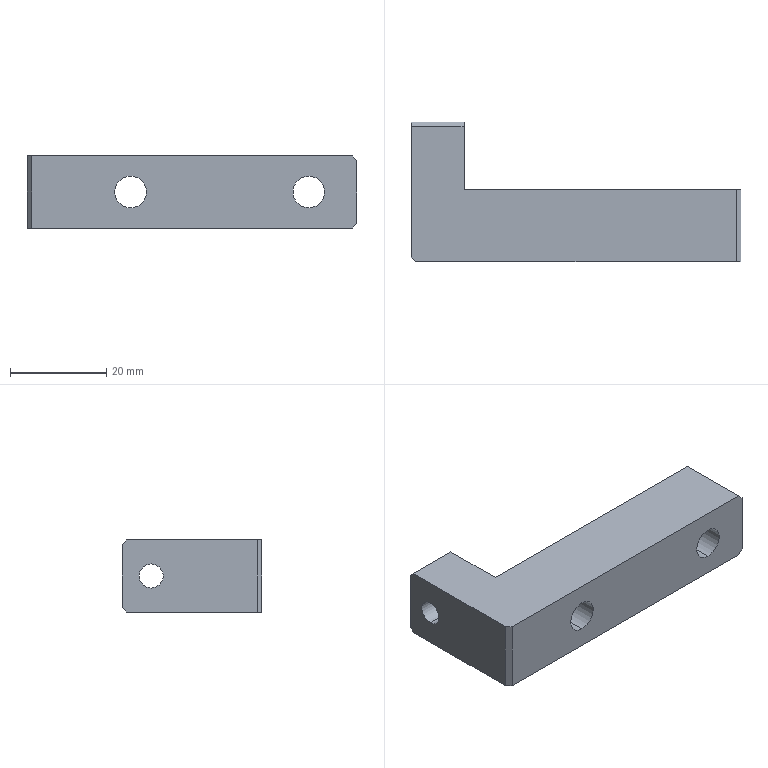Part | SolidWorks | features HoleWzd 2, Chamfer 1, Extrusion 1, ICE 1 | 1 solid | 25 faces | box 68.5 x 29 x 15 mm | volume 15619 mm3 | plane 15 | cylinder 10 | commonest cylinder face diameters 6.6 x4 11 x4 5 x2
STEP:
#1=CARTESIAN_POINT('',(-23.25,15.5,-2.5));
#2=VERTEX_POINT('',#1);
#3=CARTESIAN_POINT('',(-23.25,15.5,2.5));
#4=VERTEX_POINT('',#3);
#5=CARTESIAN_POINT('',(-23.25,15.5,0.));
#6=DIRECTION('',(-1.,0.,0.));
#7=DIRECTION('',(0.,0.,1.));
#8=AXIS2_PLACEMENT_3D('',#5,#6,#7);
#9=CIRCLE('',#8,2.5);
#10=EDGE_CURVE('',#2,#4,#9,.T.);
#11=ORIENTED_EDGE('',*,*,#10,.F.);
#12=CARTESIAN_POINT('',(-34.25,15.5,-2.5));
#13=VERTEX_POINT('',#12);
#14=CARTESIAN_POINT('',(-34.25,15.5,-2.5));
#15=DIRECTION('',(-1.,0.,0.));
#16=VECTOR('',#15,1000.);
#17=LINE('',#14,#16);
#18=EDGE_CURVE('',#2,#13,#17,.T.);
#19=ORIENTED_EDGE('',*,*,#18,.T.);
#20=CARTESIAN_POINT('',(-34.25,15.5,2.5));
#21=VERTEX_POINT('',#20);
#22=CARTESIAN_POINT('',(-34.25,15.5,0.));
#23=DIRECTION('',(-1.,0.,0.));
#24=DIRECTION('',(0.,0.,1.));
#25=AXIS2_PLACEMENT_3D('',#22,#23,#24);
#26=CIRCLE('',#25,2.5);
#27=EDGE_CURVE('',#13,#21,#26,.T.);
#28=ORIENTED_EDGE('',*,*,#27,.T.);
#29=CARTESIAN_POINT('',(-34.25,15.5,2.5));
#30=DIRECTION('',(-1.,0.,0.));
#31=VECTOR('',#30,1000.);
#32=LINE('',#29,#31);
#33=EDGE_CURVE('',#4,#21,#32,.T.);
#34=ORIENTED_EDGE('',*,*,#33,.F.);
#35=EDGE_LOOP('',(#11,#19,#28,#34));
#36=FACE_OUTER_BOUND('',#35,.T.);
#37=CARTESIAN_POINT('',(-34.25,15.5,0.));
#38=DIRECTION('',(-1.,0.,0.));
#39=DIRECTION('',(0.,0.,1.));
#40=AXIS2_PLACEMENT_3D('',#37,#38,#39);
#41=CYLINDRICAL_SURFACE('',#40,2.5);
#42=ADVANCED_FACE('',(#36),#41,.F.);
#43=CARTESIAN_POINT('',(24.25,0.7,-5.5));
#44=VERTEX_POINT('',#43);
#45=CARTESIAN_POINT('',(24.25,0.7,5.5));
#46=VERTEX_POINT('',#45);
#47=CARTESIAN_POINT('',(24.25,0.7,0.));
#48=DIRECTION('',(0.,1.,0.));
#49=DIRECTION('',(0.,0.,1.));
#50=AXIS2_PLACEMENT_3D('',#47,#48,#49);
#51=CIRCLE('',#50,5.5);
#52=EDGE_CURVE('',#44,#46,#51,.T.);
#53=ORIENTED_EDGE('',*,*,#52,.F.);
#54=CARTESIAN_POINT('',(24.25,7.5,-5.5));
#55=VERTEX_POINT('',#54);
#56=CARTESIAN_POINT('',(24.25,7.5,-5.5));
#57=DIRECTION('',(0.,1.,0.));
#58=VECTOR('',#57,1000.);
#59=LINE('',#56,#58);
#60=EDGE_CURVE('',#44,#55,#59,.T.);
#61=ORIENTED_EDGE('',*,*,#60,.T.);
#62=CARTESIAN_POINT('',(24.25,7.5,5.5));
#63=VERTEX_POINT('',#62);
#64=CARTESIAN_POINT('',(24.25,7.5,0.));
#65=DIRECTION('',(0.,1.,0.));
#66=DIRECTION('',(0.,0.,1.));
#67=AXIS2_PLACEMENT_3D('',#64,#65,#66);
#68=CIRCLE('',#67,5.5);
#69=EDGE_CURVE('',#55,#63,#68,.T.);
#70=ORIENTED_EDGE('',*,*,#69,.T.);
#71=CARTESIAN_POINT('',(24.25,7.5,5.5));
#72=DIRECTION('',(0.,1.,0.));
#73=VECTOR('',#72,1000.);
#74=LINE('',#71,#73);
#75=EDGE_CURVE('',#46,#63,#74,.T.);
#76=ORIENTED_EDGE('',*,*,#75,.F.);
#77=EDGE_LOOP('',(#53,#61,#70,#76));
#78=FACE_OUTER_BOUND('',#77,.T.);
#79=CARTESIAN_POINT('',(24.25,7.5,0.));
#80=DIRECTION('',(0.,1.,0.));
#81=DIRECTION('',(0.,0.,1.));
#82=AXIS2_PLACEMENT_3D('',#79,#80,#81);
#83=CYLINDRICAL_SURFACE('',#82,5.5);
#84=ADVANCED_FACE('',(#78),#83,.F.);
#85=CARTESIAN_POINT('',(24.25,-7.5,-3.3));
#86=VERTEX_POINT('',#85);
#87=CARTESIAN_POINT('',(24.25,-7.5,3.3));
#88=VERTEX_POINT('',#87);
#89=CARTESIAN_POINT('',(24.25,-7.5,0.));
#90=DIRECTION('',(0.,1.,0.));
#91=DIRECTION('',(0.,0.,1.));
#92=AXIS2_PLACEMENT_3D('',#89,#90,#91);
#93=CIRCLE('',#92,3.3);
#94=EDGE_CURVE('',#86,#88,#93,.T.);
#95=ORIENTED_EDGE('',*,*,#94,.F.);
#96=CARTESIAN_POINT('',(24.25,0.7,-3.3));
#97=VERTEX_POINT('',#96);
#98=CARTESIAN_POINT('',(24.25,7.5,-3.3));
#99=DIRECTION('',(0.,1.,0.));
#100=VECTOR('',#99,1000.);
#101=LINE('',#98,#100);
#102=EDGE_CURVE('',#86,#97,#101,.T.);
#103=ORIENTED_EDGE('',*,*,#102,.T.);
#104=CARTESIAN_POINT('',(24.25,0.7,3.3));
#105=VERTEX_POINT('',#104);
#106=CARTESIAN_POINT('',(24.25,0.7,0.));
#107=DIRECTION('',(0.,1.,0.));
#108=DIRECTION('',(0.,0.,1.));
#109=AXIS2_PLACEMENT_3D('',#106,#107,#108);
#110=CIRCLE('',#109,3.3);
#111=EDGE_CURVE('',#97,#105,#110,.T.);
#112=ORIENTED_EDGE('',*,*,#111,.T.);
#113=CARTESIAN_POINT('',(24.25,7.5,3.3));
#114=DIRECTION('',(0.,1.,0.));
#115=VECTOR('',#114,1000.);
#116=LINE('',#113,#115);
#117=EDGE_CURVE('',#88,#105,#116,.T.);
#118=ORIENTED_EDGE('',*,*,#117,.F.);
#119=EDGE_LOOP('',(#95,#103,#112,#118));
#120=FACE_OUTER_BOUND('',#119,.T.);
#121=CARTESIAN_POINT('',(24.25,7.5,0.));
#122=DIRECTION('',(0.,1.,0.));
#123=DIRECTION('',(0.,0.,1.));
#124=AXIS2_PLACEMENT_3D('',#121,#122,#123);
#125=CYLINDRICAL_SURFACE('',#124,3.3);
#126=ADVANCED_FACE('',(#120),#125,.F.);
#127=CARTESIAN_POINT('',(-12.75,0.7,-5.5));
#128=VERTEX_POINT('',#127);
#129=CARTESIAN_POINT('',(-12.75,0.7,5.5));
#130=VERTEX_POINT('',#129);
#131=CARTESIAN_POINT('',(-12.75,0.7,0.));
#132=DIRECTION('',(0.,1.,0.));
#133=DIRECTION('',(0.,0.,1.));
#134=AXIS2_PLACEMENT_3D('',#131,#132,#133);
#135=CIRCLE('',#134,5.5);
#136=EDGE_CURVE('',#128,#130,#135,.T.);
#137=ORIENTED_EDGE('',*,*,#136,.F.);
#138=CARTESIAN_POINT('',(-12.75,7.5,-5.5));
#139=VERTEX_POINT('',#138);
#140=CARTESIAN_POINT('',(-12.75,7.5,-5.5));
#141=DIRECTION('',(0.,1.,0.));
#142=VECTOR('',#141,1000.);
#143=LINE('',#140,#142);
#144=EDGE_CURVE('',#128,#139,#143,.T.);
#145=ORIENTED_EDGE('',*,*,#144,.T.);
#146=CARTESIAN_POINT('',(-12.75,7.5,5.5));
#147=VERTEX_POINT('',#146);
#148=CARTESIAN_POINT('',(-12.75,7.5,0.));
#149=DIRECTION('',(0.,1.,0.));
#150=DIRECTION('',(0.,0.,1.));
#151=AXIS2_PLACEMENT_3D('',#148,#149,#150);
#152=CIRCLE('',#151,5.5);
#153=EDGE_CURVE('',#139,#147,#152,.T.);
#154=ORIENTED_EDGE('',*,*,#153,.T.);
#155=CARTESIAN_POINT('',(-12.75,7.5,5.5));
#156=DIRECTION('',(0.,1.,0.));
#157=VECTOR('',#156,1000.);
#158=LINE('',#155,#157);
#159=EDGE_CURVE('',#130,#147,#158,.T.);
#160=ORIENTED_EDGE('',*,*,#159,.F.);
#161=EDGE_LOOP('',(#137,#145,#154,#160));
#162=FACE_OUTER_BOUND('',#161,.T.);
#163=CARTESIAN_POINT('',(-12.75,7.5,0.));
#164=DIRECTION('',(0.,1.,0.));
#165=DIRECTION('',(0.,0.,1.));
#166=AXIS2_PLACEMENT_3D('',#163,#164,#165);
#167=CYLINDRICAL_SURFACE('',#166,5.5);
#168=ADVANCED_FACE('',(#162),#167,.F.);
#169=CARTESIAN_POINT('',(-12.75,-7.5,-3.3));
#170=VERTEX_POINT('',#169);
#171=CARTESIAN_POINT('',(-12.75,-7.5,3.3));
#172=VERTEX_POINT('',#171);
#173=CARTESIAN_POINT('',(-12.75,-7.5,0.));
#174=DIRECTION('',(0.,1.,0.));
#175=DIRECTION('',(0.,0.,1.));
#176=AXIS2_PLACEMENT_3D('',#173,#174,#175);
#177=CIRCLE('',#176,3.3);
#178=EDGE_CURVE('',#170,#172,#177,.T.);
#179=ORIENTED_EDGE('',*,*,#178,.F.);
#180=CARTESIAN_POINT('',(-12.75,0.7,-3.3));
#181=VERTEX_POINT('',#180);
#182=CARTESIAN_POINT('',(-12.75,7.5,-3.3));
#183=DIRECTION('',(0.,1.,0.));
#184=VECTOR('',#183,1000.);
#185=LINE('',#182,#184);
#186=EDGE_CURVE('',#170,#181,#185,.T.);
#187=ORIENTED_EDGE('',*,*,#186,.T.);
#188=CARTESIAN_POINT('',(-12.75,0.7,3.3));
#189=VERTEX_POINT('',#188);
#190=CARTESIAN_POINT('',(-12.75,0.7,0.));
#191=DIRECTION('',(0.,1.,0.));
#192=DIRECTION('',(0.,0.,1.));
#193=AXIS2_PLACEMENT_3D('',#190,#191,#192);
#194=CIRCLE('',#193,3.3);
#195=EDGE_CURVE('',#181,#189,#194,.T.);
#196=ORIENTED_EDGE('',*,*,#195,.T.);
#197=CARTESIAN_POINT('',(-12.75,7.5,3.3));
#198=DIRECTION('',(0.,1.,0.));
#199=VECTOR('',#198,1000.);
#200=LINE('',#197,#199);
#201=EDGE_CURVE('',#172,#189,#200,.T.);
#202=ORIENTED_EDGE('',*,*,#201,.F.);
#203=EDGE_LOOP('',(#179,#187,#196,#202));
#204=FACE_OUTER_BOUND('',#203,.T.);
#205=CARTESIAN_POINT('',(-12.75,7.5,0.));
#206=DIRECTION('',(0.,1.,0.));
#207=DIRECTION('',(0.,0.,1.));
#208=AXIS2_PLACEMENT_3D('',#205,#206,#207);
#209=CYLINDRICAL_SURFACE('',#208,3.3);
#210=ADVANCED_FACE('',(#204),#209,.F.);
#211=CARTESIAN_POINT('',(24.25,7.5,0.));
#212=DIRECTION('',(0.,1.,0.));
#213=DIRECTION('',(0.,0.,1.));
#214=AXIS2_PLACEMENT_3D('',#211,#212,#213);
#215=CIRCLE('',#214,5.5);
#216=EDGE_CURVE('',#63,#55,#215,.T.);
#217=ORIENTED_EDGE('',*,*,#216,.F.);
#218=ORIENTED_EDGE('',*,*,#69,.F.);
#219=EDGE_LOOP('',(#217,#218));
#220=FACE_BOUND('',#219,.T.);
#221=CARTESIAN_POINT('',(-12.75,7.5,0.));
#222=DIRECTION('',(0.,1.,0.));
#223=DIRECTION('',(0.,0.,1.));
#224=AXIS2_PLACEMENT_3D('',#221,#222,#223);
#225=CIRCLE('',#224,5.5);
#226=EDGE_CURVE('',#147,#139,#225,.T.);
#227=ORIENTED_EDGE('',*,*,#226,.F.);
#228=ORIENTED_EDGE('',*,*,#153,.F.);
#229=EDGE_LOOP('',(#227,#228));
#230=FACE_BOUND('',#229,.T.);
#231=CARTESIAN_POINT('',(34.25,7.5,6.5));
#232=VERTEX_POINT('',#231);
#233=CARTESIAN_POINT('',(34.25,7.5,-6.5));
#234=VERTEX_POINT('',#233);
#235=CARTESIAN_POINT('',(34.25,7.5,7.5));
#236=DIRECTION('',(0.,0.,-1.));
#237=VECTOR('',#236,1000.);
#238=LINE('',#235,#237);
#239=EDGE_CURVE('',#232,#234,#238,.T.);
#240=ORIENTED_EDGE('',*,*,#239,.T.);
#241=CARTESIAN_POINT('',(33.25,7.5,-7.5));
#242=VERTEX_POINT('',#241);
#243=CARTESIAN_POINT('',(33.25,7.5,-7.5));
#244=DIRECTION('',(-0.7071,0.,-0.7071));
#245=VECTOR('',#244,1000.);
#246=LINE('',#243,#245);
#247=EDGE_CURVE('',#234,#242,#246,.T.);
#248=ORIENTED_EDGE('',*,*,#247,.T.);
#249=CARTESIAN_POINT('',(-23.25,7.5,-7.5));
#250=VERTEX_POINT('',#249);
#251=CARTESIAN_POINT('',(-34.25,7.5,-7.5));
#252=DIRECTION('',(-1.,0.,0.));
#253=VECTOR('',#252,1000.);
#254=LINE('',#251,#253);
#255=EDGE_CURVE('',#242,#250,#254,.T.);
#256=ORIENTED_EDGE('',*,*,#255,.T.);
#257=CARTESIAN_POINT('',(-23.25,7.5,7.5));
#258=VERTEX_POINT('',#257);
#259=CARTESIAN_POINT('',(-23.25,7.5,-7.5));
#260=DIRECTION('',(0.,0.,-1.));
#261=VECTOR('',#260,1000.);
#262=LINE('',#259,#261);
#263=EDGE_CURVE('',#258,#250,#262,.T.);
#264=ORIENTED_EDGE('',*,*,#263,.F.);
#265=CARTESIAN_POINT('',(33.25,7.5,7.5));
#266=VERTEX_POINT('',#265);
#267=CARTESIAN_POINT('',(-34.25,7.5,7.5));
#268=DIRECTION('',(1.,0.,0.));
#269=VECTOR('',#268,1000.);
#270=LINE('',#267,#269);
#271=EDGE_CURVE('',#258,#266,#270,.T.);
#272=ORIENTED_EDGE('',*,*,#271,.T.);
#273=CARTESIAN_POINT('',(34.25,7.5,6.5));
#274=DIRECTION('',(0.7071,0.,-0.7071));
#275=VECTOR('',#274,1000.);
#276=LINE('',#273,#275);
#277=EDGE_CURVE('',#266,#232,#276,.T.);
#278=ORIENTED_EDGE('',*,*,#277,.T.);
#279=EDGE_LOOP('',(#240,#248,#256,#264,#272,#278));
#280=FACE_OUTER_BOUND('',#279,.T.);
#281=CARTESIAN_POINT('',(0.,7.5,0.));
#282=DIRECTION('',(0.,-1.,0.));
#283=DIRECTION('',(0.,0.,-1.));
#284=AXIS2_PLACEMENT_3D('',#281,#282,#283);
#285=PLANE('',#284);
#286=ADVANCED_FACE('',(#220,#230,#280),#285,.F.);
#287=CARTESIAN_POINT('',(34.25,-7.5,6.5));
#288=VERTEX_POINT('',#287);
#289=CARTESIAN_POINT('',(34.25,-7.5,-6.5));
#290=VERTEX_POINT('',#289);
#291=CARTESIAN_POINT('',(34.25,-7.5,7.5));
#292=DIRECTION('',(0.,0.,-1.));
#293=VECTOR('',#292,1000.);
#294=LINE('',#291,#293);
#295=EDGE_CURVE('',#288,#290,#294,.T.);
#296=ORIENTED_EDGE('',*,*,#295,.T.);
#297=CARTESIAN_POINT('',(34.25,7.5,-6.5));
#298=DIRECTION('',(0.,1.,0.));
#299=VECTOR('',#298,1000.);
#300=LINE('',#297,#299);
#301=EDGE_CURVE('',#290,#234,#300,.T.);
#302=ORIENTED_EDGE('',*,*,#301,.T.);
#303=ORIENTED_EDGE('',*,*,#239,.F.);
#304=CARTESIAN_POINT('',(34.25,7.5,6.5));
#305=DIRECTION('',(0.,-1.,0.));
#306=VECTOR('',#305,1000.);
#307=LINE('',#304,#306);
#308=EDGE_CURVE('',#232,#288,#307,.T.);
#309=ORIENTED_EDGE('',*,*,#308,.T.);
#310=EDGE_LOOP('',(#296,#302,#303,#309));
#311=FACE_OUTER_BOUND('',#310,.T.);
#312=CARTESIAN_POINT('',(34.25,7.5,7.5));
#313=DIRECTION('',(-1.,0.,0.));
#314=DIRECTION('',(0.,0.,1.));
#315=AXIS2_PLACEMENT_3D('',#312,#313,#314);
#316=PLANE('',#315);
#317=ADVANCED_FACE('',(#311),#316,.F.);
#318=ORIENTED_EDGE('',*,*,#255,.F.);
#319=CARTESIAN_POINT('',(33.25,-7.5,-7.5));
#320=VERTEX_POINT('',#319);
#321=CARTESIAN_POINT('',(33.25,7.5,-7.5));
#322=DIRECTION('',(0.,-1.,0.));
#323=VECTOR('',#322,1000.);
#324=LINE('',#321,#323);
#325=EDGE_CURVE('',#242,#320,#324,.T.);
#326=ORIENTED_EDGE('',*,*,#325,.T.);
#327=CARTESIAN_POINT('',(-33.25,-7.5,-7.5));
#328=VERTEX_POINT('',#327);
#329=CARTESIAN_POINT('',(-34.25,-7.5,-7.5));
#330=DIRECTION('',(-1.,0.,0.));
#331=VECTOR('',#330,1000.);
#332=LINE('',#329,#331);
#333=EDGE_CURVE('',#320,#328,#332,.T.);
#334=ORIENTED_EDGE('',*,*,#333,.T.);
#335=CARTESIAN_POINT('',(-34.25,-6.5,-7.5));
#336=VERTEX_POINT('',#335);
#337=CARTESIAN_POINT('',(-34.25,-6.5,-7.5));
#338=DIRECTION('',(-0.7071,0.7071,0.));
#339=VECTOR('',#338,1000.);
#340=LINE('',#337,#339);
#341=EDGE_CURVE('',#328,#336,#340,.T.);
#342=ORIENTED_EDGE('',*,*,#341,.T.);
#343=CARTESIAN_POINT('',(-34.25,20.5,-7.5));
#344=VERTEX_POINT('',#343);
#345=CARTESIAN_POINT('',(-34.25,7.5,-7.5));
#346=DIRECTION('',(0.,-1.,0.));
#347=VECTOR('',#346,1000.);
#348=LINE('',#345,#347);
#349=EDGE_CURVE('',#344,#336,#348,.T.);
#350=ORIENTED_EDGE('',*,*,#349,.F.);
#351=CARTESIAN_POINT('',(-23.25,20.5,-7.5));
#352=VERTEX_POINT('',#351);
#353=CARTESIAN_POINT('',(-23.25,20.5,-7.5));
#354=DIRECTION('',(1.,0.,0.));
#355=VECTOR('',#354,1000.);
#356=LINE('',#353,#355);
#357=EDGE_CURVE('',#344,#352,#356,.T.);
#358=ORIENTED_EDGE('',*,*,#357,.T.);
#359=CARTESIAN_POINT('',(-23.25,21.5,-7.5));
#360=DIRECTION('',(0.,-1.,0.));
#361=VECTOR('',#360,1000.);
#362=LINE('',#359,#361);
#363=EDGE_CURVE('',#352,#250,#362,.T.);
#364=ORIENTED_EDGE('',*,*,#363,.T.);
#365=EDGE_LOOP('',(#318,#326,#334,#342,#350,#358,#364));
#366=FACE_OUTER_BOUND('',#365,.T.);
#367=CARTESIAN_POINT('',(-34.25,7.5,-7.5));
#368=DIRECTION('',(0.,0.,1.));
#369=DIRECTION('',(1.,0.,0.));
#370=AXIS2_PLACEMENT_3D('',#367,#368,#369);
#371=PLANE('',#370);
#372=ADVANCED_FACE('',(#366),#371,.F.);
#373=CARTESIAN_POINT('',(-34.25,15.5,0.));
#374=DIRECTION('',(-1.,0.,0.));
#375=DIRECTION('',(0.,0.,1.));
#376=AXIS2_PLACEMENT_3D('',#373,#374,#375);
#377=CIRCLE('',#376,2.5);
#378=EDGE_CURVE('',#21,#13,#377,.T.);
#379=ORIENTED_EDGE('',*,*,#378,.F.);
#380=ORIENTED_EDGE('',*,*,#27,.F.);
#381=EDGE_LOOP('',(#379,#380));
#382=FACE_BOUND('',#381,.T.);
#383=ORIENTED_EDGE('',*,*,#349,.T.);
#384=CARTESIAN_POINT('',(-34.25,-6.5,7.5));
#385=VERTEX_POINT('',#384);
#386=CARTESIAN_POINT('',(-34.25,-6.5,7.5));
#387=DIRECTION('',(0.,0.,1.));
#388=VECTOR('',#387,1000.);
#389=LINE('',#386,#388);
#390=EDGE_CURVE('',#336,#385,#389,.T.);
#391=ORIENTED_EDGE('',*,*,#390,.T.);
#392=CARTESIAN_POINT('',(-34.25,20.5,7.5));
#393=VERTEX_POINT('',#392);
#394=CARTESIAN_POINT('',(-34.25,7.5,7.5));
#395=DIRECTION('',(0.,-1.,0.));
#396=VECTOR('',#395,1000.);
#397=LINE('',#394,#396);
#398=EDGE_CURVE('',#393,#385,#397,.T.);
#399=ORIENTED_EDGE('',*,*,#398,.F.);
#400=CARTESIAN_POINT('',(-34.25,21.5,6.5));
#401=VERTEX_POINT('',#400);
#402=CARTESIAN_POINT('',(-34.25,21.5,6.5));
#403=DIRECTION('',(0.,0.7071,-0.7071));
#404=VECTOR('',#403,1000.);
#405=LINE('',#402,#404);
#406=EDGE_CURVE('',#393,#401,#405,.T.);
#407=ORIENTED_EDGE('',*,*,#406,.T.);
#408=CARTESIAN_POINT('',(-34.25,21.5,-6.5));
#409=VERTEX_POINT('',#408);
#410=CARTESIAN_POINT('',(-34.25,21.5,-7.5));
#411=DIRECTION('',(0.,0.,1.));
#412=VECTOR('',#411,1000.);
#413=LINE('',#410,#412);
#414=EDGE_CURVE('',#409,#401,#413,.T.);
#415=ORIENTED_EDGE('',*,*,#414,.F.);
#416=CARTESIAN_POINT('',(-34.25,21.5,-6.5));
#417=DIRECTION('',(0.,-0.7071,-0.7071));
#418=VECTOR('',#417,1000.);
#419=LINE('',#416,#418);
#420=EDGE_CURVE('',#409,#344,#419,.T.);
#421=ORIENTED_EDGE('',*,*,#420,.T.);
#422=EDGE_LOOP('',(#383,#391,#399,#407,#415,#421));
#423=FACE_OUTER_BOUND('',#422,.T.);
#424=CARTESIAN_POINT('',(-34.25,7.5,7.5));
#425=DIRECTION('',(1.,0.,0.));
#426=DIRECTION('',(0.,0.,-1.));
#427=AXIS2_PLACEMENT_3D('',#424,#425,#426);
#428=PLANE('',#427);
#429=ADVANCED_FACE('',(#382,#423),#428,.F.);
#430=CARTESIAN_POINT('',(-33.25,-7.5,7.5));
#431=VERTEX_POINT('',#430);
#432=CARTESIAN_POINT('',(33.25,-7.5,7.5));
#433=VERTEX_POINT('',#432);
#434=CARTESIAN_POINT('',(-34.25,-7.5,7.5));
#435=DIRECTION('',(1.,0.,0.));
#436=VECTOR('',#435,1000.);
#437=LINE('',#434,#436);
#438=EDGE_CURVE('',#431,#433,#437,.T.);
#439=ORIENTED_EDGE('',*,*,#438,.T.);
#440=CARTESIAN_POINT('',(33.25,7.5,7.5));
#441=DIRECTION('',(0.,1.,0.));
#442=VECTOR('',#441,1000.);
#443=LINE('',#440,#442);
#444=EDGE_CURVE('',#433,#266,#443,.T.);
#445=ORIENTED_EDGE('',*,*,#444,.T.);
#446=ORIENTED_EDGE('',*,*,#271,.F.);
#447=CARTESIAN_POINT('',(-23.25,20.5,7.5));
#448=VERTEX_POINT('',#447);
#449=CARTESIAN_POINT('',(-23.25,21.5,7.5));
#450=DIRECTION('',(0.,-1.,0.));
#451=VECTOR('',#450,1000.);
#452=LINE('',#449,#451);
#453=EDGE_CURVE('',#448,#258,#452,.T.);
#454=ORIENTED_EDGE('',*,*,#453,.F.);
#455=CARTESIAN_POINT('',(-34.25,20.5,7.5));
#456=DIRECTION('',(-1.,0.,0.));
#457=VECTOR('',#456,1000.);
#458=LINE('',#455,#457);
#459=EDGE_CURVE('',#448,#393,#458,.T.);
#460=ORIENTED_EDGE('',*,*,#459,.T.);
#461=ORIENTED_EDGE('',*,*,#398,.T.);
#462=CARTESIAN_POINT('',(-34.25,-6.5,7.5));
#463=DIRECTION('',(0.7071,-0.7071,0.));
#464=VECTOR('',#463,1000.);
#465=LINE('',#462,#464);
#466=EDGE_CURVE('',#385,#431,#465,.T.);
#467=ORIENTED_EDGE('',*,*,#466,.T.);
#468=EDGE_LOOP('',(#439,#445,#446,#454,#460,#461,#467));
#469=FACE_OUTER_BOUND('',#468,.T.);
#470=CARTESIAN_POINT('',(-34.25,7.5,7.5));
#471=DIRECTION('',(0.,0.,-1.));
#472=DIRECTION('',(-1.,0.,0.));
#473=AXIS2_PLACEMENT_3D('',#470,#471,#472);
#474=PLANE('',#473);
#475=ADVANCED_FACE('',(#469),#474,.F.);
#476=CARTESIAN_POINT('',(24.25,-7.5,0.));
#477=DIRECTION('',(0.,1.,0.));
#478=DIRECTION('',(0.,0.,1.));
#479=AXIS2_PLACEMENT_3D('',#476,#477,#478);
#480=CIRCLE('',#479,3.3);
#481=EDGE_CURVE('',#88,#86,#480,.T.);
#482=ORIENTED_EDGE('',*,*,#481,.T.);
#483=ORIENTED_EDGE('',*,*,#94,.T.);
#484=EDGE_LOOP('',(#482,#483));
#485=FACE_BOUND('',#484,.T.);
#486=CARTESIAN_POINT('',(-12.75,-7.5,0.));
#487=DIRECTION('',(0.,1.,0.));
#488=DIRECTION('',(0.,0.,1.));
#489=AXIS2_PLACEMENT_3D('',#486,#487,#488);
#490=CIRCLE('',#489,3.3);
#491=EDGE_CURVE('',#172,#170,#490,.T.);
#492=ORIENTED_EDGE('',*,*,#491,.T.);
#493=ORIENTED_EDGE('',*,*,#178,.T.);
#494=EDGE_LOOP('',(#492,#493));
#495=FACE_BOUND('',#494,.T.);
#496=ORIENTED_EDGE('',*,*,#333,.F.);
#497=CARTESIAN_POINT('',(20.375,-7.5,-20.375));
#498=DIRECTION('',(0.7071,0.,0.7071));
#499=VECTOR('',#498,1000.);
#500=LINE('',#497,#499);
#501=EDGE_CURVE('',#320,#290,#500,.T.);
#502=ORIENTED_EDGE('',*,*,#501,.T.);
#503=ORIENTED_EDGE('',*,*,#295,.F.);
#504=CARTESIAN_POINT('',(20.375,-7.5,20.375));
#505=DIRECTION('',(-0.7071,0.,0.7071));
#506=VECTOR('',#505,1000.);
#507=LINE('',#504,#506);
#508=EDGE_CURVE('',#288,#433,#507,.T.);
#509=ORIENTED_EDGE('',*,*,#508,.T.);
#510=ORIENTED_EDGE('',*,*,#438,.F.);
#511=CARTESIAN_POINT('',(-33.25,-7.5,-7.5));
#512=DIRECTION('',(0.,0.,-1.));
#513=VECTOR('',#512,1000.);
#514=LINE('',#511,#513);
#515=EDGE_CURVE('',#431,#328,#514,.T.);
#516=ORIENTED_EDGE('',*,*,#515,.T.);
#517=EDGE_LOOP('',(#496,#502,#503,#509,#510,#516));
#518=FACE_OUTER_BOUND('',#517,.T.);
#519=CARTESIAN_POINT('',(0.,-7.5,0.));
#520=DIRECTION('',(0.,-1.,0.));
#521=DIRECTION('',(0.,0.,-1.));
#522=AXIS2_PLACEMENT_3D('',#519,#520,#521);
#523=PLANE('',#522);
#524=ADVANCED_FACE('',(#485,#495,#518),#523,.T.);
#525=CARTESIAN_POINT('',(-23.25,15.5,0.));
#526=DIRECTION('',(-1.,0.,0.));
#527=DIRECTION('',(0.,0.,1.));
#528=AXIS2_PLACEMENT_3D('',#525,#526,#527);
#529=CIRCLE('',#528,2.5);
#530=EDGE_CURVE('',#4,#2,#529,.T.);
#531=ORIENTED_EDGE('',*,*,#530,.T.);
#532=ORIENTED_EDGE('',*,*,#10,.T.);
#533=EDGE_LOOP('',(#531,#532));
#534=FACE_BOUND('',#533,.T.);
#535=ORIENTED_EDGE('',*,*,#363,.F.);
#536=CARTESIAN_POINT('',(-23.25,21.5,-6.5));
#537=VERTEX_POINT('',#536);
#538=CARTESIAN_POINT('',(-23.25,21.5,-6.5));
#539=DIRECTION('',(0.,0.7071,0.7071));
#540=VECTOR('',#539,1000.);
#541=LINE('',#538,#540);
#542=EDGE_CURVE('',#352,#537,#541,.T.);
#543=ORIENTED_EDGE('',*,*,#542,.T.);
#544=CARTESIAN_POINT('',(-23.25,21.5,6.5));
#545=VERTEX_POINT('',#544);
#546=CARTESIAN_POINT('',(-23.25,21.5,-7.5));
#547=DIRECTION('',(0.,0.,-1.));
#548=VECTOR('',#547,1000.);
#549=LINE('',#546,#548);
#550=EDGE_CURVE('',#545,#537,#549,.T.);
#551=ORIENTED_EDGE('',*,*,#550,.F.);
#552=CARTESIAN_POINT('',(-23.25,21.5,6.5));
#553=DIRECTION('',(0.,-0.7071,0.7071));
#554=VECTOR('',#553,1000.);
#555=LINE('',#552,#554);
#556=EDGE_CURVE('',#545,#448,#555,.T.);
#557=ORIENTED_EDGE('',*,*,#556,.T.);
#558=ORIENTED_EDGE('',*,*,#453,.T.);
#559=ORIENTED_EDGE('',*,*,#263,.T.);
#560=EDGE_LOOP('',(#535,#543,#551,#557,#558,#559));
#561=FACE_OUTER_BOUND('',#560,.T.);
#562=CARTESIAN_POINT('',(-23.25,21.5,-7.5));
#563=DIRECTION('',(-1.,0.,0.));
#564=DIRECTION('',(0.,0.,1.));
#565=AXIS2_PLACEMENT_3D('',#562,#563,#564);
#566=PLANE('',#565);
#567=ADVANCED_FACE('',(#534,#561),#566,.F.);
#568=ORIENTED_EDGE('',*,*,#550,.T.);
#569=CARTESIAN_POINT('',(-34.25,21.5,-6.5));
#570=DIRECTION('',(-1.,0.,0.));
#571=VECTOR('',#570,1000.);
#572=LINE('',#569,#571);
#573=EDGE_CURVE('',#537,#409,#572,.T.);
#574=ORIENTED_EDGE('',*,*,#573,.T.);
#575=ORIENTED_EDGE('',*,*,#414,.T.);
#576=CARTESIAN_POINT('',(-23.25,21.5,6.5));
#577=DIRECTION('',(1.,0.,0.));
#578=VECTOR('',#577,1000.);
#579=LINE('',#576,#578);
#580=EDGE_CURVE('',#401,#545,#579,.T.);
#581=ORIENTED_EDGE('',*,*,#580,.T.);
#582=EDGE_LOOP('',(#568,#574,#575,#581));
#583=FACE_OUTER_BOUND('',#582,.T.);
#584=CARTESIAN_POINT('',(0.,21.5,0.));
#585=DIRECTION('',(0.,1.,0.));
#586=DIRECTION('',(0.,0.,1.));
#587=AXIS2_PLACEMENT_3D('',#584,#585,#586);
#588=PLANE('',#587);
#589=ADVANCED_FACE('',(#583),#588,.T.);
#590=ORIENTED_EDGE('',*,*,#247,.F.);
#591=ORIENTED_EDGE('',*,*,#301,.F.);
#592=ORIENTED_EDGE('',*,*,#501,.F.);
#593=ORIENTED_EDGE('',*,*,#325,.F.);
#594=EDGE_LOOP('',(#590,#591,#592,#593));
#595=FACE_OUTER_BOUND('',#594,.T.);
#596=CARTESIAN_POINT('',(33.25,7.5,-7.5));
#597=DIRECTION('',(-0.7071,0.,0.7071));
#598=DIRECTION('',(0.,-1.,0.));
#599=AXIS2_PLACEMENT_3D('',#596,#597,#598);
#600=PLANE('',#599);
#601=ADVANCED_FACE('',(#595),#600,.F.);
#602=ORIENTED_EDGE('',*,*,#277,.F.);
#603=ORIENTED_EDGE('',*,*,#444,.F.);
#604=ORIENTED_EDGE('',*,*,#508,.F.);
#605=ORIENTED_EDGE('',*,*,#308,.F.);
#606=EDGE_LOOP('',(#602,#603,#604,#605));
#607=FACE_OUTER_BOUND('',#606,.T.);
#608=CARTESIAN_POINT('',(34.25,7.5,6.5));
#609=DIRECTION('',(-0.7071,0.,-0.7071));
#610=DIRECTION('',(0.,-1.,0.));
#611=AXIS2_PLACEMENT_3D('',#608,#609,#610);
#612=PLANE('',#611);
#613=ADVANCED_FACE('',(#607),#612,.F.);
#614=ORIENTED_EDGE('',*,*,#341,.F.);
#615=ORIENTED_EDGE('',*,*,#515,.F.);
#616=ORIENTED_EDGE('',*,*,#466,.F.);
#617=ORIENTED_EDGE('',*,*,#390,.F.);
#618=EDGE_LOOP('',(#614,#615,#616,#617));
#619=FACE_OUTER_BOUND('',#618,.T.);
#620=CARTESIAN_POINT('',(-34.25,-6.5,7.5));
#621=DIRECTION('',(-0.7071,-0.7071,0.));
#622=DIRECTION('',(0.,0.,-1.));
#623=AXIS2_PLACEMENT_3D('',#620,#621,#622);
#624=PLANE('',#623);
#625=ADVANCED_FACE('',(#619),#624,.T.);
#626=ORIENTED_EDGE('',*,*,#542,.F.);
#627=ORIENTED_EDGE('',*,*,#357,.F.);
#628=ORIENTED_EDGE('',*,*,#420,.F.);
#629=ORIENTED_EDGE('',*,*,#573,.F.);
#630=EDGE_LOOP('',(#626,#627,#628,#629));
#631=FACE_OUTER_BOUND('',#630,.T.);
#632=CARTESIAN_POINT('',(0.,21.5,-6.5));
#633=DIRECTION('',(0.,0.7071,-0.7071));
#634=DIRECTION('',(1.,0.,0.));
#635=AXIS2_PLACEMENT_3D('',#632,#633,#634);
#636=PLANE('',#635);
#637=ADVANCED_FACE('',(#631),#636,.T.);
#638=ORIENTED_EDGE('',*,*,#406,.F.);
#639=ORIENTED_EDGE('',*,*,#459,.F.);
#640=ORIENTED_EDGE('',*,*,#556,.F.);
#641=ORIENTED_EDGE('',*,*,#580,.F.);
#642=EDGE_LOOP('',(#638,#639,#640,#641));
#643=FACE_OUTER_BOUND('',#642,.T.);
#644=CARTESIAN_POINT('',(0.,21.5,6.5));
#645=DIRECTION('',(0.,0.7071,0.7071));
#646=DIRECTION('',(-1.,0.,0.));
#647=AXIS2_PLACEMENT_3D('',#644,#645,#646);
#648=PLANE('',#647);
#649=ADVANCED_FACE('',(#643),#648,.T.);
#650=ORIENTED_EDGE('',*,*,#186,.F.);
#651=ORIENTED_EDGE('',*,*,#491,.F.);
#652=ORIENTED_EDGE('',*,*,#201,.T.);
#653=CARTESIAN_POINT('',(-12.75,0.7,0.));
#654=DIRECTION('',(0.,1.,0.));
#655=DIRECTION('',(0.,0.,1.));
#656=AXIS2_PLACEMENT_3D('',#653,#654,#655);
#657=CIRCLE('',#656,3.3);
#658=EDGE_CURVE('',#189,#181,#657,.T.);
#659=ORIENTED_EDGE('',*,*,#658,.T.);
#660=EDGE_LOOP('',(#650,#651,#652,#659));
#661=FACE_OUTER_BOUND('',#660,.T.);
#662=CARTESIAN_POINT('',(-12.75,7.5,0.));
#663=DIRECTION('',(0.,1.,0.));
#664=DIRECTION('',(0.,0.,1.));
#665=AXIS2_PLACEMENT_3D('',#662,#663,#664);
#666=CYLINDRICAL_SURFACE('',#665,3.3);
#667=ADVANCED_FACE('',(#661),#666,.F.);
#668=ORIENTED_EDGE('',*,*,#658,.F.);
#669=ORIENTED_EDGE('',*,*,#195,.F.);
#670=EDGE_LOOP('',(#668,#669));
#671=FACE_BOUND('',#670,.T.);
#672=CARTESIAN_POINT('',(-12.75,0.7,0.));
#673=DIRECTION('',(0.,1.,0.));
#674=DIRECTION('',(0.,0.,1.));
#675=AXIS2_PLACEMENT_3D('',#672,#673,#674);
#676=CIRCLE('',#675,5.5);
#677=EDGE_CURVE('',#130,#128,#676,.T.);
#678=ORIENTED_EDGE('',*,*,#677,.T.);
#679=ORIENTED_EDGE('',*,*,#136,.T.);
#680=EDGE_LOOP('',(#678,#679));
#681=FACE_OUTER_BOUND('',#680,.T.);
#682=CARTESIAN_POINT('',(-9.45,0.7,0.));
#683=DIRECTION('',(0.,-1.,0.));
#684=DIRECTION('',(0.,0.,-1.));
#685=AXIS2_PLACEMENT_3D('',#682,#683,#684);
#686=PLANE('',#685);
#687=ADVANCED_FACE('',(#671,#681),#686,.F.);
#688=ORIENTED_EDGE('',*,*,#144,.F.);
#689=ORIENTED_EDGE('',*,*,#677,.F.);
#690=ORIENTED_EDGE('',*,*,#159,.T.);
#691=ORIENTED_EDGE('',*,*,#226,.T.);
#692=EDGE_LOOP('',(#688,#689,#690,#691));
#693=FACE_OUTER_BOUND('',#692,.T.);
#694=CARTESIAN_POINT('',(-12.75,7.5,0.));
#695=DIRECTION('',(0.,1.,0.));
#696=DIRECTION('',(0.,0.,1.));
#697=AXIS2_PLACEMENT_3D('',#694,#695,#696);
#698=CYLINDRICAL_SURFACE('',#697,5.5);
#699=ADVANCED_FACE('',(#693),#698,.F.);
#700=ORIENTED_EDGE('',*,*,#102,.F.);
#701=ORIENTED_EDGE('',*,*,#481,.F.);
#702=ORIENTED_EDGE('',*,*,#117,.T.);
#703=CARTESIAN_POINT('',(24.25,0.7,0.));
#704=DIRECTION('',(0.,1.,0.));
#705=DIRECTION('',(0.,0.,1.));
#706=AXIS2_PLACEMENT_3D('',#703,#704,#705);
#707=CIRCLE('',#706,3.3);
#708=EDGE_CURVE('',#105,#97,#707,.T.);
#709=ORIENTED_EDGE('',*,*,#708,.T.);
#710=EDGE_LOOP('',(#700,#701,#702,#709));
#711=FACE_OUTER_BOUND('',#710,.T.);
#712=CARTESIAN_POINT('',(24.25,7.5,0.));
#713=DIRECTION('',(0.,1.,0.));
#714=DIRECTION('',(0.,0.,1.));
#715=AXIS2_PLACEMENT_3D('',#712,#713,#714);
#716=CYLINDRICAL_SURFACE('',#715,3.3);
#717=ADVANCED_FACE('',(#711),#716,.F.);
#718=ORIENTED_EDGE('',*,*,#708,.F.);
#719=ORIENTED_EDGE('',*,*,#111,.F.);
#720=EDGE_LOOP('',(#718,#719));
#721=FACE_BOUND('',#720,.T.);
#722=CARTESIAN_POINT('',(24.25,0.7,0.));
#723=DIRECTION('',(0.,1.,0.));
#724=DIRECTION('',(0.,0.,1.));
#725=AXIS2_PLACEMENT_3D('',#722,#723,#724);
#726=CIRCLE('',#725,5.5);
#727=EDGE_CURVE('',#46,#44,#726,.T.);
#728=ORIENTED_EDGE('',*,*,#727,.T.);
#729=ORIENTED_EDGE('',*,*,#52,.T.);
#730=EDGE_LOOP('',(#728,#729));
#731=FACE_OUTER_BOUND('',#730,.T.);
#732=CARTESIAN_POINT('',(27.55,0.7,0.));
#733=DIRECTION('',(0.,-1.,0.));
#734=DIRECTION('',(0.,0.,-1.));
#735=AXIS2_PLACEMENT_3D('',#732,#733,#734);
#736=PLANE('',#735);
#737=ADVANCED_FACE('',(#721,#731),#736,.F.);
#738=ORIENTED_EDGE('',*,*,#60,.F.);
#739=ORIENTED_EDGE('',*,*,#727,.F.);
#740=ORIENTED_EDGE('',*,*,#75,.T.);
#741=ORIENTED_EDGE('',*,*,#216,.T.);
#742=EDGE_LOOP('',(#738,#739,#740,#741));
#743=FACE_OUTER_BOUND('',#742,.T.);
#744=CARTESIAN_POINT('',(24.25,7.5,0.));
#745=DIRECTION('',(0.,1.,0.));
#746=DIRECTION('',(0.,0.,1.));
#747=AXIS2_PLACEMENT_3D('',#744,#745,#746);
#748=CYLINDRICAL_SURFACE('',#747,5.5);
#749=ADVANCED_FACE('',(#743),#748,.F.);
#750=ORIENTED_EDGE('',*,*,#18,.F.);
#751=ORIENTED_EDGE('',*,*,#530,.F.);
#752=ORIENTED_EDGE('',*,*,#33,.T.);
#753=ORIENTED_EDGE('',*,*,#378,.T.);
#754=EDGE_LOOP('',(#750,#751,#752,#753));
#755=FACE_OUTER_BOUND('',#754,.T.);
#756=CARTESIAN_POINT('',(-34.25,15.5,0.));
#757=DIRECTION('',(-1.,0.,0.));
#758=DIRECTION('',(0.,0.,1.));
#759=AXIS2_PLACEMENT_3D('',#756,#757,#758);
#760=CYLINDRICAL_SURFACE('',#759,2.5);
#761=ADVANCED_FACE('',(#755),#760,.F.);
#762=CLOSED_SHELL('',(#42,#84,#126,#168,#210,#286,#317,#372,#429,#475,#524,#567,#589,#601,#613,#625,#637,#649,#667,#687,#699,#717,#737,#749,#761));
#763=MANIFOLD_SOLID_BREP('',#762);
#764=CARTESIAN_POINT('',(0.,0.,0.));
#765=DIRECTION('',(0.,0.,1.));
#766=DIRECTION('',(1.,0.,0.));
#767=AXIS2_PLACEMENT_3D('',#764,#765,#766);
#768=(LENGTH_UNIT()NAMED_UNIT(*)SI_UNIT(.MILLI.,.METRE.));
#769=UNCERTAINTY_MEASURE_WITH_UNIT(LENGTH_MEASURE(0.00001),#768,'','');
#770=(NAMED_UNIT(*)PLANE_ANGLE_UNIT()SI_UNIT($,.RADIAN.));
#771=(NAMED_UNIT(*)SI_UNIT($,.STERADIAN.)SOLID_ANGLE_UNIT());
#772=(GEOMETRIC_REPRESENTATION_CONTEXT(3)GLOBAL_UNCERTAINTY_ASSIGNED_CONTEXT((#769))GLOBAL_UNIT_ASSIGNED_CONTEXT((#768,#770,#771))REPRESENTATION_CONTEXT('',''));
#773=ADVANCED_BREP_SHAPE_REPRESENTATION('',(#763,#767),#772);